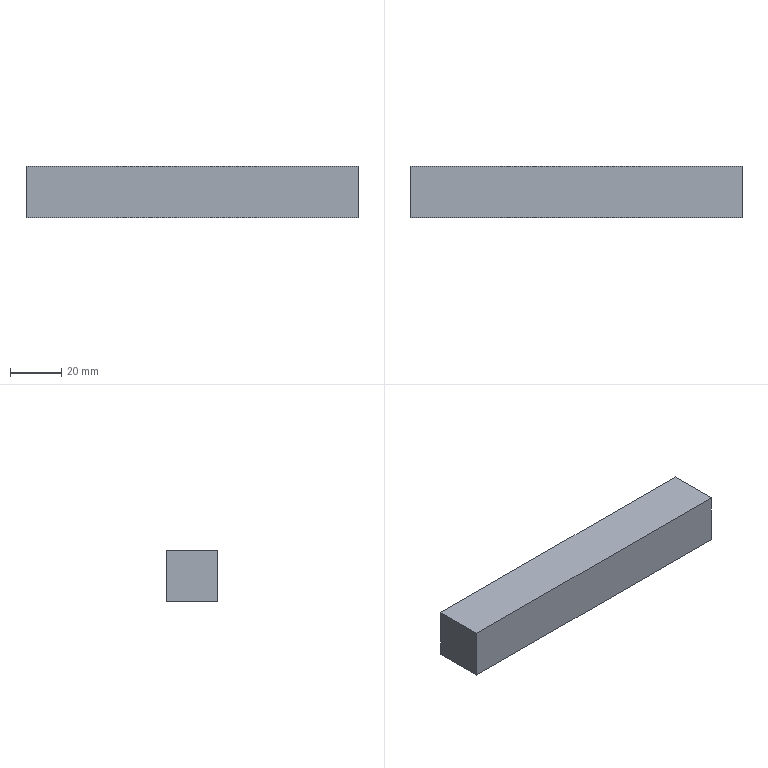Part | NX | features solid 2 | 1 solid | 6 faces | box 130 x 20 x 20 mm | volume 52000 mm3 | plane 6
STEP:
#1=CARTESIAN_POINT('',(-240.,50.,-20.));
#2=VERTEX_POINT('',#1);
#3=CARTESIAN_POINT('',(-240.,70.,-20.));
#4=VERTEX_POINT('',#3);
#5=CARTESIAN_POINT('',(-240.,50.,-20.));
#6=DIRECTION('',(0.,-1.,0.));
#7=VECTOR('',#6,1000.);
#8=LINE('',#5,#7);
#9=EDGE_CURVE('',#2,#4,#8,.F.);
#10=ORIENTED_EDGE('',*,*,#9,.T.);
#11=CARTESIAN_POINT('',(-240.,70.,-40.));
#12=VERTEX_POINT('',#11);
#13=CARTESIAN_POINT('',(-240.,70.,-40.));
#14=DIRECTION('',(0.,0.,-1.));
#15=VECTOR('',#14,1000.);
#16=LINE('',#13,#15);
#17=EDGE_CURVE('',#12,#4,#16,.F.);
#18=ORIENTED_EDGE('',*,*,#17,.F.);
#19=CARTESIAN_POINT('',(-240.,50.,-40.));
#20=VERTEX_POINT('',#19);
#21=CARTESIAN_POINT('',(-240.,40.,-40.));
#22=DIRECTION('',(0.,1.,0.));
#23=VECTOR('',#22,1000.);
#24=LINE('',#21,#23);
#25=EDGE_CURVE('',#20,#12,#24,.T.);
#26=ORIENTED_EDGE('',*,*,#25,.F.);
#27=CARTESIAN_POINT('',(-240.,50.,-40.));
#28=DIRECTION('',(0.,0.,-1.));
#29=VECTOR('',#28,1000.);
#30=LINE('',#27,#29);
#31=EDGE_CURVE('',#20,#2,#30,.F.);
#32=ORIENTED_EDGE('',*,*,#31,.T.);
#33=EDGE_LOOP('',(#10,#18,#26,#32));
#34=FACE_BOUND('',#33,.T.);
#35=CARTESIAN_POINT('',(-240.,40.,-20.));
#36=DIRECTION('',(1.,0.,0.));
#37=DIRECTION('',(0.,-1.,0.));
#38=AXIS2_PLACEMENT_3D('',#35,#36,#37);
#39=PLANE('',#38);
#40=ADVANCED_FACE('',(#34),#39,.F.);
#41=ORIENTED_EDGE('',*,*,#25,.T.);
#42=CARTESIAN_POINT('',(-110.,70.,-40.));
#43=VERTEX_POINT('',#42);
#44=CARTESIAN_POINT('',(-165.,70.,-40.));
#45=DIRECTION('',(-1.,0.,0.));
#46=VECTOR('',#45,1000.);
#47=LINE('',#44,#46);
#48=EDGE_CURVE('',#12,#43,#47,.F.);
#49=ORIENTED_EDGE('',*,*,#48,.T.);
#50=CARTESIAN_POINT('',(-110.,50.,-40.));
#51=VERTEX_POINT('',#50);
#52=CARTESIAN_POINT('',(-110.,50.,-40.));
#53=DIRECTION('',(0.,1.,0.));
#54=VECTOR('',#53,1000.);
#55=LINE('',#52,#54);
#56=EDGE_CURVE('',#51,#43,#55,.T.);
#57=ORIENTED_EDGE('',*,*,#56,.F.);
#58=CARTESIAN_POINT('',(-165.,50.,-40.));
#59=DIRECTION('',(1.,0.,0.));
#60=VECTOR('',#59,1000.);
#61=LINE('',#58,#60);
#62=EDGE_CURVE('',#20,#51,#61,.T.);
#63=ORIENTED_EDGE('',*,*,#62,.F.);
#64=EDGE_LOOP('',(#41,#49,#57,#63));
#65=FACE_BOUND('',#64,.T.);
#66=CARTESIAN_POINT('',(-165.,50.,-40.));
#67=DIRECTION('',(0.,0.,1.));
#68=DIRECTION('',(1.,0.,0.));
#69=AXIS2_PLACEMENT_3D('',#66,#67,#68);
#70=PLANE('',#69);
#71=ADVANCED_FACE('',(#65),#70,.F.);
#72=ORIENTED_EDGE('',*,*,#56,.T.);
#73=CARTESIAN_POINT('',(-110.,70.,-20.));
#74=VERTEX_POINT('',#73);
#75=CARTESIAN_POINT('',(-110.,70.,-20.));
#76=DIRECTION('',(0.,0.,-1.));
#77=VECTOR('',#76,1000.);
#78=LINE('',#75,#77);
#79=EDGE_CURVE('',#43,#74,#78,.F.);
#80=ORIENTED_EDGE('',*,*,#79,.T.);
#81=CARTESIAN_POINT('',(-110.,50.,-20.));
#82=VERTEX_POINT('',#81);
#83=CARTESIAN_POINT('',(-110.,40.,-20.));
#84=DIRECTION('',(0.,-1.,0.));
#85=VECTOR('',#84,1000.);
#86=LINE('',#83,#85);
#87=EDGE_CURVE('',#82,#74,#86,.F.);
#88=ORIENTED_EDGE('',*,*,#87,.F.);
#89=CARTESIAN_POINT('',(-110.,50.,-20.));
#90=DIRECTION('',(0.,0.,-1.));
#91=VECTOR('',#90,1000.);
#92=LINE('',#89,#91);
#93=EDGE_CURVE('',#51,#82,#92,.F.);
#94=ORIENTED_EDGE('',*,*,#93,.F.);
#95=EDGE_LOOP('',(#72,#80,#88,#94));
#96=FACE_BOUND('',#95,.T.);
#97=CARTESIAN_POINT('',(-110.,40.,-20.));
#98=DIRECTION('',(-1.,0.,0.));
#99=DIRECTION('',(0.,-1.,0.));
#100=AXIS2_PLACEMENT_3D('',#97,#98,#99);
#101=PLANE('',#100);
#102=ADVANCED_FACE('',(#96),#101,.F.);
#103=CARTESIAN_POINT('',(-165.,50.,-20.));
#104=DIRECTION('',(1.,0.,0.));
#105=VECTOR('',#104,1000.);
#106=LINE('',#103,#105);
#107=EDGE_CURVE('',#2,#82,#106,.T.);
#108=ORIENTED_EDGE('',*,*,#107,.T.);
#109=ORIENTED_EDGE('',*,*,#87,.T.);
#110=CARTESIAN_POINT('',(-165.,70.,-20.));
#111=DIRECTION('',(-1.,0.,0.));
#112=VECTOR('',#111,1000.);
#113=LINE('',#110,#112);
#114=EDGE_CURVE('',#4,#74,#113,.F.);
#115=ORIENTED_EDGE('',*,*,#114,.F.);
#116=ORIENTED_EDGE('',*,*,#9,.F.);
#117=EDGE_LOOP('',(#108,#109,#115,#116));
#118=FACE_BOUND('',#117,.T.);
#119=CARTESIAN_POINT('',(-165.,50.,-20.));
#120=DIRECTION('',(0.,0.,1.));
#121=DIRECTION('',(1.,0.,0.));
#122=AXIS2_PLACEMENT_3D('',#119,#120,#121);
#123=PLANE('',#122);
#124=ADVANCED_FACE('',(#118),#123,.T.);
#125=ORIENTED_EDGE('',*,*,#79,.F.);
#126=ORIENTED_EDGE('',*,*,#48,.F.);
#127=ORIENTED_EDGE('',*,*,#17,.T.);
#128=ORIENTED_EDGE('',*,*,#114,.T.);
#129=EDGE_LOOP('',(#125,#126,#127,#128));
#130=FACE_BOUND('',#129,.T.);
#131=CARTESIAN_POINT('',(-165.,70.,-40.));
#132=DIRECTION('',(0.,-1.,0.));
#133=DIRECTION('',(0.,0.,-1.));
#134=AXIS2_PLACEMENT_3D('',#131,#132,#133);
#135=PLANE('',#134);
#136=ADVANCED_FACE('',(#130),#135,.F.);
#137=ORIENTED_EDGE('',*,*,#93,.T.);
#138=ORIENTED_EDGE('',*,*,#107,.F.);
#139=ORIENTED_EDGE('',*,*,#31,.F.);
#140=ORIENTED_EDGE('',*,*,#62,.T.);
#141=EDGE_LOOP('',(#137,#138,#139,#140));
#142=FACE_BOUND('',#141,.T.);
#143=CARTESIAN_POINT('',(-165.,50.,-40.));
#144=DIRECTION('',(0.,-1.,0.));
#145=DIRECTION('',(0.,0.,-1.));
#146=AXIS2_PLACEMENT_3D('',#143,#144,#145);
#147=PLANE('',#146);
#148=ADVANCED_FACE('',(#142),#147,.T.);
#149=CLOSED_SHELL('',(#40,#71,#102,#124,#136,#148));
#150=MANIFOLD_SOLID_BREP('',#149);
#151=(LENGTH_UNIT()NAMED_UNIT(*)SI_UNIT(.MILLI.,.METRE.));
#152=UNCERTAINTY_MEASURE_WITH_UNIT(LENGTH_MEASURE(0.00001),#151,'','');
#153=(NAMED_UNIT(*)PLANE_ANGLE_UNIT()SI_UNIT($,.RADIAN.));
#154=(NAMED_UNIT(*)SI_UNIT($,.STERADIAN.)SOLID_ANGLE_UNIT());
#155=(GEOMETRIC_REPRESENTATION_CONTEXT(3)GLOBAL_UNCERTAINTY_ASSIGNED_CONTEXT((#152))GLOBAL_UNIT_ASSIGNED_CONTEXT((#151,#153,#154))REPRESENTATION_CONTEXT('',''));
#156=ADVANCED_BREP_SHAPE_REPRESENTATION('',(#150),#155);